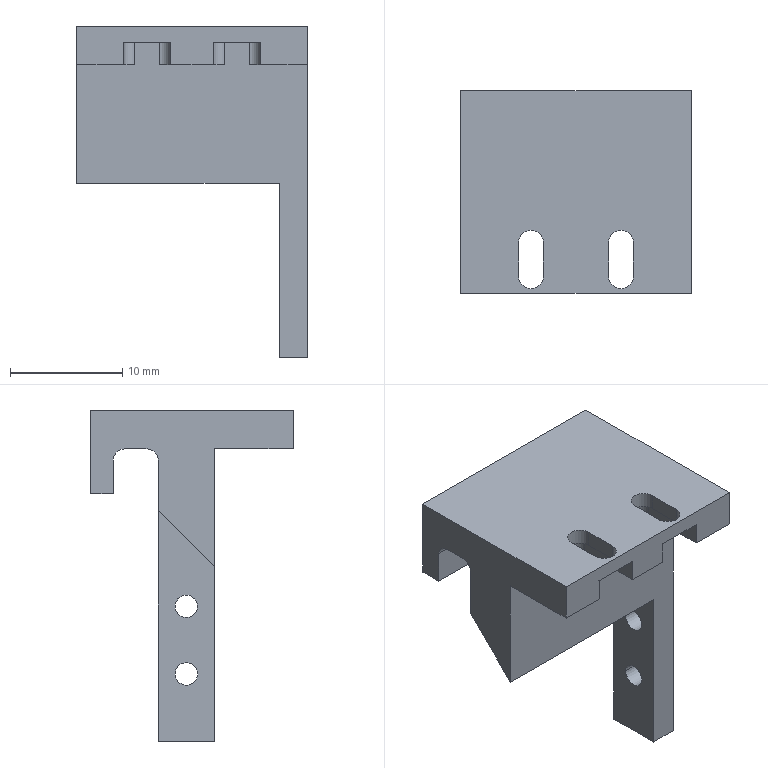NC program | NX | posted with a generic post | part box 20.5 x 18 x 29.4 mm
Lines 1922 to 2950 of 6588:
(CAVITY_MILL_COPY_COPY , TOOL : D2)
N3830 T02 M6
N3832 G54
N3834 G17 G0 G90 X-3.982 Y0.408 S7500 M3
N3836 G43 Z30. H2
N3838 Z-14.1
N3840 G94 G1 Z-15.6 F1000.
N3842 X-4.3 Y0.323
N3844 G2 X-5.266 Y0.581 R1.
N3846 X-6.258 Y2.485 R3.56 F850.
N3848 G3 X-6.75 Y2.899 R0.5
N3850 G1 Y-0.9
N3852 X-2.946
N3854 G3 X-3.361 Y-0.407 R0.5
N3856 G2 X-5.266 Y0.581 R3.56
N3858 X-5.526 Y1.547 R1.
N3860 G1 X-5.441 Y1.865
N3862 Z-14.1
N3864 G0 X-3.931 Y0.484 Z-14.2
N3866 G1 Z-15.7 F1000.
N3868 X-4.247 Y0.392
N3870 G2 X-5.218 Y0.631 R1.
N3872 X-6.258 Y2.57 R3.56 F850.
N3874 G3 X-6.75 Y2.982 R0.5
N3876 G1 Y-0.8
N3878 X-2.949
N3880 G3 X-3.364 Y-0.307 R0.5
N3882 G2 X-5.218 Y0.631 R3.56
N3884 X-5.497 Y1.591 R1.
N3886 G1 X-5.419 Y1.911
N3888 Z-14.2
N3890 G0 X-3.881 Y0.561 Z-14.3
N3892 G1 Z-15.8 F1000.
N3894 X-4.196 Y0.463
N3896 G2 X-5.171 Y0.682 R1.
N3898 X-6.258 Y2.646 R3.56 F850.
N3900 G3 X-6.751 Y3.055 R0.5
N3902 G1 X-6.75 Y3.
N3904 Y-0.7
N3906 X-2.954
N3908 G3 X-3.369 Y-0.207 R0.5
N3910 G2 X-5.171 Y0.682 R3.56
N3912 X-5.469 Y1.637 R1.
N3914 G1 X-5.397 Y1.958
N3916 Z-14.3
N3918 G0 X-3.833 Y0.639 Z-14.4
N3920 G1 Z-15.9 F1000.
N3922 X-4.145 Y0.535
N3924 G2 X-5.125 Y0.734 R1.
N3926 X-6.259 Y2.714 R3.56 F850.
N3928 G3 X-6.757 Y3.118 R0.5
N3930 G1 X-6.75 Y3.
N3932 Y-0.6
N3934 X-2.961
N3936 G3 X-3.376 Y-0.107 R0.5
N3938 G2 X-5.125 Y0.734 R3.56
N3940 X-5.443 Y1.682 R1.
N3942 G1 X-5.377 Y2.005
N3944 Z-14.4
N3946 G0 X-3.786 Y0.718 Z-14.5
N3948 G1 Z-16. F1000.
N3950 X-4.097 Y0.607
N3952 G2 X-5.08 Y0.787 R1.
N3954 X-6.26 Y2.775 R3.56 F850.
N3956 G3 X-6.765 Y3.173 R0.5
N3958 G1 X-6.75 Y3.
N3960 Y-0.5
N3962 X-2.97
N3964 G3 X-3.385 Y-0.007 R0.5
N3966 G2 X-5.08 Y0.787 R3.56
N3968 X-5.416 Y1.729 R1.
N3970 G1 X-5.357 Y2.053
N3972 Z-14.5
N3974 G0 X-3.741 Y0.798 Z-14.6
N3976 G1 Z-16.1 F1000.
N3978 X-4.049 Y0.681
N3980 G2 X-5.036 Y0.841 R1.
N3982 X-6.262 Y2.83 R3.56 F850.
N3984 G3 X-6.775 Y3.221 R0.5
N3986 G2 X-6.75 Y3. R1.
N3988 G1 Y-0.4
N3990 X-2.982
N3992 G3 X-3.396 Y0.093 R0.5
N3994 G2 X-5.036 Y0.841 R3.56
N3996 X-5.391 Y1.776 R1.
N3998 G1 X-5.339 Y2.101
N4000 Z-14.6
N4002 G0 X-3.697 Y0.88 Z-14.7
N4004 G1 Z-16.2 F1000.
N4006 X-4.003 Y0.756
N4008 G2 X-4.993 Y0.896 R1.
N4010 X-6.263 Y2.88 R3.56 F850.
N4012 G3 X-6.785 Y3.263 R0.5
N4014 G2 X-6.75 Y3. R1.
N4016 G1 Y-0.3
N4018 X-2.995
N4020 G3 X-3.409 Y0.193 R0.5
N4022 G2 X-4.993 Y0.896 R3.56
N4024 X-5.367 Y1.824 R1.
N4026 G1 X-5.321 Y2.15
N4028 Z-14.7
N4030 G0 X-3.655 Y0.962 Z-14.8
N4032 G1 Z-16.3 F1000.
N4034 X-3.958 Y0.833
N4036 G2 X-4.951 Y0.952 R1.
N4038 X-6.265 Y2.925 R3.56 F850.
N4040 G3 X-6.796 Y3.3 R0.5
N4042 G2 X-6.75 Y3. R1.
N4044 G1 Y-0.2
N4046 X-3.01
N4048 G3 X-3.424 Y0.293 R0.5
N4050 G2 X-4.951 Y0.952 R3.56
N4052 X-5.344 Y1.872 R1.
N4054 G1 X-5.304 Y2.199
N4056 Z-14.8
N4058 G0 X-3.615 Y1.045 Z-14.9
N4060 G1 Z-16.4 F1000.
N4062 X-3.915 Y0.91
N4064 G2 X-4.91 Y1.01 R1.
N4066 X-6.267 Y2.968 R3.56 F850.
N4068 G3 X-6.807 Y3.334 R0.5
N4070 G2 X-6.75 Y3. R1.
N4072 G1 Y-0.1
N4074 X-3.027
N4076 G3 X-3.441 Y0.393 R0.5
N4078 G2 X-4.91 Y1.01 R3.56
N4080 X-5.321 Y1.921 R1.
N4082 G1 X-5.288 Y2.249
N4084 Z-14.9
N4086 G0 X-3.576 Y1.13 Z-15.
N4088 G1 Z-16.5 F1000.
N4090 X-3.873 Y0.988
N4092 G2 X-4.87 Y1.068 R1.
N4094 X-6.27 Y3.007 R3.56 F850.
N4096 G3 X-6.818 Y3.363 R0.5
N4098 G2 X-6.75 Y3. R1.
N4100 G1 Y0.
N4102 X-3.046
N4104 G3 X-3.461 Y0.493 R0.5
N4106 G2 X-4.87 Y1.068 R3.56
N4108 X-5.3 Y1.971 R1.
N4110 G1 X-5.273 Y2.299
N4112 Z-15.
N4114 G0 X-3.538 Y1.216 Z-15.1
N4116 G1 Z-16.6 F1000.
N4118 X-3.833 Y1.068
N4120 G2 X-4.831 Y1.127 R1.
N4122 X-6.272 Y3.045 R3.56 F850.
N4124 G3 X-6.829 Y3.39 R0.5
N4126 G2 X-6.75 Y3. R1.
N4128 G1 Y0.1
N4130 X-3.068
N4132 G3 X-3.482 Y0.593 R0.5
N4134 G2 X-4.831 Y1.127 R3.56
N4136 X-5.279 Y2.021 R1.
N4138 G1 X-5.26 Y2.35
N4140 Z-15.1
N4142 G0 X-3.502 Y1.303 Z-15.2
N4144 G1 Z-16.7 F1000.
N4146 X-3.794 Y1.149
N4148 G2 X-4.793 Y1.187 R1.
N4150 X-6.275 Y3.08 R3.56 F850.
N4152 G3 X-6.84 Y3.415 R0.5
N4154 G2 X-6.75 Y3. R1.
N4156 G1 Y0.2
N4158 X-3.092
N4160 G3 X-3.506 Y0.693 R0.5
N4162 G2 X-4.793 Y1.187 R3.56
N4164 X-5.259 Y2.072 R1.
N4166 G1 X-5.247 Y2.401
N4168 Z-15.2
N4170 G0 X-3.468 Y1.391 Z-15.3
N4172 G1 Z-16.8 F1000.
N4174 X-3.756 Y1.231
N4176 G2 X-4.756 Y1.249 R1.
N4178 X-6.279 Y3.114 R3.56 F850.
N4180 G3 X-6.851 Y3.437 R0.5
N4182 G2 X-6.75 Y3. R1.
N4184 G1 Y0.3
N4186 X-3.117
N4188 G3 X-3.532 Y0.793 R0.5
N4190 G2 X-4.756 Y1.249 R3.56
N4192 X-5.241 Y2.123 R1.
N4194 G1 X-5.235 Y2.453
N4196 Z-15.3
N4198 G0 X-3.436 Y1.48 Z-15.4
N4200 G1 Z-16.9 F1000.
N4202 X-3.72 Y1.314
N4204 G2 X-4.72 Y1.311 R1.
N4206 X-6.282 Y3.147 R3.56 F850.
N4208 G3 X-6.861 Y3.458 R0.5
N4210 G2 X-6.75 Y3. R1.
N4212 G1 Y0.4
N4214 X-3.145
N4216 G3 X-3.56 Y0.893 R0.5
N4218 G2 X-4.72 Y1.311 R3.56
N4220 X-5.223 Y2.176 R1.
N4222 G1 X-5.224 Y2.505
N4224 Z-15.4
N4226 G0 X-3.41 Y1.567 Z-15.5
N4228 G1 Z-17. F1000.
N4230 X-3.686 Y1.399
N4232 G2 X-4.685 Y1.375 R1.
N4234 X-6.286 Y3.178 R3.56 F850.
N4236 G3 X-6.871 Y3.477 R0.5
N4238 G2 X-6.75 Y3. R1.
N4240 G1 Y0.5
N4242 X-3.176
N4244 G3 X-3.59 Y0.993 R0.5
N4246 G2 X-4.685 Y1.375 R3.56
N4248 X-5.206 Y2.229 R1.
N4250 G1 X-5.214 Y2.558
N4252 Z-15.5
N4254 G0 X-3.39 Y1.653 Z-15.6
N4256 G1 Z-17.1 F1000.
N4258 X-3.653 Y1.485
N4260 G2 X-4.652 Y1.44 R1.
N4262 X-6.29 Y3.209 R3.56 F850.
N4264 G3 X-6.882 Y3.496 R0.5
N4266 G2 X-6.75 Y3. R1.
N4268 G1 Y0.6
N4270 X-3.208
N4272 G3 X-3.623 Y1.093 R0.5
N4274 G2 X-4.652 Y1.44 R3.56
N4276 X-5.19 Y2.282 R1.
N4278 G1 X-5.205 Y2.611
N4280 Z-15.6
N4282 G0 X-3.376 Y1.737 Z-15.7
N4284 G1 Z-17.2 F1000.
N4286 X-3.622 Y1.572
N4288 G2 X-4.619 Y1.506 R1.
N4290 X-6.295 Y3.24 R3.56 F850.
N4292 G3 X-6.892 Y3.514 R0.5
N4294 G2 X-6.75 Y3. R1.
N4296 G1 Y0.7
N4298 X-3.243
N4300 G3 X-3.658 Y1.193 R0.5
N4302 G2 X-4.619 Y1.506 R3.56
N4304 X-5.176 Y2.337 R1.
N4306 G1 X-5.198 Y2.665
N4308 Z-15.7
N4310 G0 X-3.366 Y1.819 Z-15.8
N4312 G1 Z-17.3 F1000.
N4314 X-3.592 Y1.66
N4316 G2 X-4.588 Y1.573 R1.
N4318 X-6.3 Y3.271 R3.56 F850.
N4320 G3 X-6.903 Y3.532 R0.5
N4322 G2 X-6.75 Y3. R1.
N4324 G1 Y0.8
N4326 X-3.281
N4328 G3 X-3.695 Y1.293 R0.5
N4330 G2 X-4.588 Y1.573 R3.56
N4332 X-5.162 Y2.392 R1.
N4334 G1 X-5.191 Y2.72
N4336 Z-15.8
N4338 G0 X-3.361 Y1.899 Z-15.9
N4340 G1 Z-17.4 F1000.
N4342 X-3.564 Y1.75
N4344 G2 X-4.558 Y1.641 R1.
N4346 X-6.306 Y3.302 R3.56 F850.
N4348 G3 X-6.915 Y3.55 R0.5
N4350 G2 X-6.75 Y3. R1.
N4352 G1 Y0.9
N4354 X-3.32
N4356 G3 X-3.735 Y1.393 R0.5
N4358 G2 X-4.558 Y1.641 R3.56
N4360 X-5.15 Y2.447 R1.
N4362 G1 X-5.185 Y2.775
N4364 Z-15.9
N4366 G0 X-3.36 Y1.978 Z-16.
N4368 G1 Z-17.5 F1000.
N4370 X-3.538 Y1.841
N4372 G2 X-4.529 Y1.711 R1.
N4374 X-6.313 Y3.333 R3.56 F850.
N4376 G3 X-6.927 Y3.568 R0.5
N4378 G2 X-6.75 Y3. R1.
N4380 G1 Y1.
N4382 X-3.363
N4384 G3 X-3.777 Y1.493 R0.5
N4386 G2 X-4.529 Y1.711 R3.56
N4388 X-5.138 Y2.504 R1.
N4390 G1 X-5.181 Y2.831
N4392 Z-16.
N4394 G0 X-3.362 Y2.055 Z-16.1
N4396 G1 Z-17.6 F1000.
N4398 X-3.513 Y1.934
N4400 G2 X-4.502 Y1.782 R1.
N4402 X-6.321 Y3.365 R3.56 F850.
N4404 G3 X-6.94 Y3.586 R0.5
N4406 G2 X-6.75 Y3. R1.
N4408 G1 Y1.1
N4410 X-3.408
N4412 G3 X-3.822 Y1.593 R0.5
N4414 G2 X-4.502 Y1.782 R3.56
N4416 X-5.128 Y2.561 R1.
N4418 G1 X-5.178 Y2.887
N4420 Z-16.1
N4422 G0 X-3.369 Y2.131 Z-16.2
N4424 G1 Z-17.7 F1000.
N4426 X-3.491 Y2.028
N4428 G2 X-4.475 Y1.854 R1.
N4430 X-6.329 Y3.396 R3.56 F850.
N4432 G3 X-6.953 Y3.604 R0.5
N4434 G2 X-6.75 Y3. R1.
N4436 G1 Y1.2
N4438 X-3.455
N4440 G3 X-3.87 Y1.693 R0.5
N4442 G2 X-4.475 Y1.854 R3.56
N4444 X-5.119 Y2.62 R1.
N4446 G1 X-5.176 Y2.944
N4448 Z-16.2
N4450 G0 X-3.379 Y2.204 Z-16.3
N4452 G1 Z-17.8 F1000.
N4454 X-3.47 Y2.124
N4456 G2 X-4.45 Y1.927 R1.
N4458 X-6.338 Y3.428 R3.56 F850.
N4460 G3 X-6.967 Y3.622 R0.5
N4462 G2 X-6.75 Y3. R1.
N4464 G1 Y1.3
N4466 X-3.506
N4468 G3 X-3.92 Y1.793 R0.5
N4470 G2 X-4.45 Y1.927 R3.56
N4472 X-5.111 Y2.679 R1.
N4474 G1 X-5.175 Y3.001
N4476 Z-16.3
N4478 G0 X-3.392 Y2.275 Z-16.4
N4480 G1 Z-17.9 F1000.
N4482 X-3.451 Y2.221
N4484 G2 X-4.427 Y2.003 R1.
N4486 X-6.348 Y3.46 R3.56 F850.
N4488 G3 X-6.981 Y3.639 R0.5
N4490 G2 X-6.75 Y3. R1.
N4492 G1 Y1.4
N4494 X-3.559
N4496 G3 X-3.973 Y1.893 R0.5
N4498 G2 X-4.427 Y2.003 R3.56
N4500 X-5.104 Y2.738 R1.
N4502 G1 X-5.176 Y3.06
N4504 Z-16.4
N4506 G0 X-3.41 Y2.344 Z-16.5
N4508 G1 Z-18. F1000.
N4510 X-3.434 Y2.32
N4512 G2 X-4.405 Y2.079 R1.
N4514 X-6.359 Y3.492 R3.56 F850.
N4516 G3 X-6.996 Y3.657 R0.5
N4518 G2 X-6.75 Y3. R1.
N4520 G1 Y1.5
N4522 X-3.615
N4524 G3 X-4.03 Y1.993 R0.5
N4526 G2 X-4.405 Y2.079 R3.56
N4528 X-5.099 Y2.799 R1.
N4530 G1 X-5.178 Y3.119
N4532 Z-16.5
N4534 G0 X-3.43 Y2.41 Z-16.6
N4536 G1 Z-18.1 F1000.
N4538 G2 X-4.384 Y2.157 R1.
N4540 X-6.371 Y3.524 R3.56 F850.
N4542 G3 X-7.011 Y3.674 R0.5
N4544 G2 X-6.75 Y3. R1.
N4546 G1 Y1.6
N4548 X-3.675
N4550 G3 X-4.089 Y2.093 R0.5
N4552 G2 X-4.384 Y2.157 R3.56
N4554 X-5.095 Y2.861 R1.
N4556 G1 X-5.182 Y3.179
N4558 Z-16.6
N4560 G0 X-3.456 Y2.475 Z-16.7
N4562 G1 Z-18.2 F1000.
N4564 G2 X-4.366 Y2.237 R1.
N4566 X-6.384 Y3.556 R3.56 F850.
N4568 G3 X-7.028 Y3.691 R0.5
N4570 G2 X-6.75 Y3. R1.
N4572 G1 Y1.7
N4574 X-3.737
N4576 G3 X-4.151 Y2.193 R0.5
N4578 G2 X-4.366 Y2.237 R3.56
N4580 X-5.092 Y2.923 R1.
N4582 G1 X-5.187 Y3.239
N4584 Z-16.7
N4586 G0 X-3.488 Y2.538 Z-16.8
N4588 G1 Z-18.3 F1000.
N4590 G2 X-4.348 Y2.318 R1.
N4592 X-6.398 Y3.589 R3.56 F850.
N4594 G3 X-7.044 Y3.709 R0.5
N4596 G2 X-6.75 Y3. R1.
N4598 G1 Y1.8
N4600 X-3.803
N4602 G3 X-4.217 Y2.293 R0.5
N4604 G1 X-4.348 Y2.318
N4606 G2 X-5.091 Y2.987 R1.
N4608 G1 X-5.193 Y3.3
N4610 Z-16.8
N4612 G0 X-3.525 Y2.602 Z-16.9
N4614 G1 Z-18.4 F1000.
N4616 G2 X-4.333 Y2.401 R1.
N4618 X-6.412 Y3.622 R3.56 F850.
N4620 G3 X-7.062 Y3.726 R0.5
N4622 G2 X-6.75 Y3. R1.
N4624 G1 Y1.9
N4626 X-3.872
N4628 G3 X-4.333 Y2.401 R0.502
N4630 G2 X-5.092 Y3.052 R1.
N4632 G1 X-5.201 Y3.363
N4634 Z-16.9
N4636 G0 X-3.503 Y2.6 Z-17.
N4638 G1 Z-18.5 F1000.
N4640 G2 X-4.31 Y2.481 R1.
N4642 G1 X-4.36 Y2.493 F850.
N4644 G2 X-6.428 Y3.655 R3.56
N4646 G3 X-7.08 Y3.742 R0.5
N4648 G2 X-6.75 Y3. R1.
N4650 G1 Y2.
N4652 X-3.945
N4654 G3 X-4.31 Y2.481 R0.5
N4656 G2 X-5.008 Y3.197 R1.
N4658 G1 X-5.044 Y3.338
N4660 Z-17.
N4662 G0 X-3.033 Y2.7 Z-17.1
N4664 G1 Z-18.6 F1000.
N4666 X-3.279 Y2.552
N4668 G2 X-4.279 Y2.537 R1.
N4670 G1 X-4.437 Y2.593 F850.
N4672 G2 X-6.445 Y3.688 R3.56
N4674 G3 X-7.099 Y3.759 R0.5
N4676 G2 X-6.75 Y3. R1.
N4678 G1 Y2.1
N4680 X-4.022
N4682 G3 X-4.279 Y2.537 R0.5
N4684 G2 X-4.787 Y3.3 R1.
N4686 G1 Z-17.1
N4688 G0 X-7.487 Y4.578 Z-17.2
N4690 G1 Z-18.7 F1000.
N4692 G3 X-7.119 Y3.776 R1.
N4694 G2 X-6.75 Y3. R1. F850.
N4696 G1 Y2.2
N4698 X-4.104
N4700 G3 X-3.238 Y2.7 R1.
N4702 G1 X-3.18 Y2.8
N4704 Z-17.2
N4706 G0 X-7.529 Y4.585 Z-17.3
N4708 G1 Z-18.8 F1000.
N4710 G3 X-7.139 Y3.792 R1.
N4712 G2 X-6.75 Y3. R1. F850.
N4714 G1 Y2.3
N4716 X-4.189
N4718 G3 X-3.323 Y2.8 R1.
N4720 G1 X-3.265 Y2.9
N4722 Z-17.3
N4724 G0 X-7.571 Y4.59 Z-17.4
N4726 G1 Z-18.9 F1000.
N4728 G3 X-7.161 Y3.808 R1.
N4730 G2 X-6.75 Y3. R1. F850.
N4732 G1 Y2.4
N4734 X-4.279
N4736 G3 X-3.413 Y2.9 R1.
N4738 G1 X-3.356 Y3.
N4740 Z-17.4
N4742 G0 X-7.615 Y4.594 Z-17.5
N4744 G1 Z-19. F1000.
N4746 G3 X-7.183 Y3.824 R1.
N4748 G2 X-6.75 Y3. R1. F850.
N4750 G1 Y2.5
N4752 X-4.375
N4754 G3 X-3.509 Y3. R1.
N4756 G1 X-3.451 Y3.1
N4758 Z-17.5
N4760 G0 X-7.661 Y4.598 Z-17.6
N4762 G1 Z-19.1 F1000.
N4764 G3 X-7.207 Y3.84 R1.
N4766 G2 X-6.75 Y3. R1. F850.
N4768 G1 Y2.6
N4770 X-4.476
N4772 G3 X-3.61 Y3.1 R1.
N4774 G1 X-3.552 Y3.2
N4776 Z-17.6
N4778 G0 X-7.708 Y4.599 Z-17.7
N4780 G1 Z-19.2 F1000.
N4782 G3 X-7.232 Y3.855 R1.
N4784 G2 X-6.75 Y3. R1. F850.
N4786 G1 Y2.7
N4788 X-4.582
N4790 G3 X-3.716 Y3.2 R1.
N4792 G1 X-3.659 Y3.3
N4794 Z-17.7
N4796 G0 X-7.756 Y4.6 Z-17.8
N4798 G1 Z-19.3 F1000.
N4800 G3 X-7.258 Y3.871 R1.
N4802 G2 X-6.75 Y3. R1. F850.
N4804 G1 Y2.8
N4806 X-4.696
N4808 G3 X-3.83 Y3.3 R1.
N4810 G1 X-3.772 Y3.4
N4812 Z-17.8
N4814 G0 X-7.806 Y4.6 Z-17.9
N4816 G1 Z-19.4 F1000.
N4818 G3 X-7.286 Y3.886 R1.
N4820 G2 X-6.75 Y3. R1. F850.
N4822 G1 Y2.9
N4824 X-4.817
N4826 G3 X-3.95 Y3.4 R1.
N4828 G1 X-3.893 Y3.5
N4830 Z-17.9
N4832 G0 X-7.859 Y4.6 Z-18.
N4834 G1 Z-19.5 F1000.
N4836 G3 X-7.315 Y3.9 R1.
N4838 G2 X-6.75 Y3. R1. F850.
N4840 G1 X-4.945
N4842 G3 X-4.079 Y3.5 R1.
N4844 G1 X-4.022 Y3.6
N4846 Z-18.
N4848 G0 X-7.915 Y4.6 Z-18.1
N4850 G1 Z-19.6 F1000.
N4852 G3 X-7.346 Y3.915 R1.
N4854 G2 X-6.755 Y3.1 R1. F850.
N4856 G1 X-5.084
N4858 G3 X-4.218 Y3.6 R1.
N4860 G1 X-4.16 Y3.7
N4862 Z-18.1
N4864 G0 X-7.974 Y4.6 Z-18.2
N4866 G1 Z-19.7 F1000.
N4868 G3 X-7.379 Y3.929 R1.
N4870 G2 X-6.77 Y3.2 R1. F850.
N4872 G1 X-5.232
N4874 G3 X-4.366 Y3.7 R1.
N4876 G1 X-4.309 Y3.8
N4878 Z-18.2
N4880 G0 X-8.037 Y4.6 Z-18.3
N4882 G1 Z-19.8 F1000.
N4884 G3 X-7.414 Y3.942 R1.
N4886 G2 X-6.796 Y3.3 R1. F850.
N4888 G1 X-5.394
N4890 G3 X-4.528 Y3.8 R1.
N4892 G1 X-4.47 Y3.9
N4894 Z-18.3
N4896 G0 X-8.106 Y4.6 Z-18.4
N4898 G1 Z-19.9 F1000.
N4900 G3 X-7.453 Y3.955 R1.
N4902 G2 X-6.833 Y3.4 R1. F850.
N4904 G1 X-5.571
N4906 G3 X-4.705 Y3.9 R1.
N4908 G1 X-4.647 Y4.
N4910 Z-18.4
N4912 G0 X-8.182 Y4.6 Z-18.5
N4914 G1 Z-20. F1000.
N4916 G3 X-7.495 Y3.967 R1.
N4918 G2 X-6.884 Y3.5 R1. F850.
N4920 G1 X-5.766
N4922 G3 X-4.9 Y4. R1.
N4924 G1 X-4.842 Y4.1
N4926 Z-18.5
N4928 G0 X-8.268 Y4.6 Z-18.6
N4930 G1 Z-20.1 F1000.
N4932 G3 X-7.542 Y3.978 R1.
N4934 G2 X-6.95 Y3.6 R1. F850.
N4936 G1 X-5.986
N4938 G3 X-5.12 Y4.1 R1.
N4940 G1 X-5.062 Y4.2
N4942 Z-18.6
N4944 G0 X-8.368 Y4.6 Z-18.7
N4946 G1 Z-20.2 F1000.
N4948 G3 X-7.596 Y3.988 R1.
N4950 G2 X-7.036 Y3.7 R1. F850.
N4952 G1 X-6.24
N4954 G3 X-5.374 Y4.2 R1.
N4956 G1 X-5.316 Y4.3
N4958 Z-18.7
N4960 G0 X-8.489 Y4.6 Z-18.8
N4962 G1 Z-20.3 F1000.
N4964 X-8.477 Y4.572
N4966 G3 X-7.659 Y3.996 R1.
N4968 G2 X-7.15 Y3.8 R1. F850.
N4970 G1 X-6.545
N4972 G3 X-5.679 Y4.3 R1.
N4974 G1 X-5.622 Y4.4
N4976 Z-18.8
N4978 G0 Z30.
N4980 X-12.055 Y3.971
N4982 Z-20.6
N4984 G1 Z-22.1 F1000.
N4986 X-11.773 Y4.134
N4988 G3 X-11.273 Y5. R1.
N4990 G1 X-10.373
N4992 X-10.374 Y4.896 F850.
N4994 X-10.25 Y4.9
N4996 X10.25
N4998 X10.374 Y4.896
N5000 G2 X10.374 Y5.104 R4.46
N5002 G1 X10.25 Y5.1
N5004 X-10.25
N5006 X-10.374 Y5.104
N5008 X-10.373 Y5.
N5010 X-11.273
N5012 G2 X-11.471 Y3.827 R3.56
N5014 G3 X-11.226 Y3.217 R0.5
N5016 G2 X-10.25 Y4. R1.
N5018 G1 X10.25
N5020 G2 X11.226 Y3.217 R1.
N5022 G3 X11.471 Y3.827 R0.5
N5024 G2 X11.471 Y6.173 R3.56
N5026 G3 X11.226 Y6.783 R0.5
N5028 G2 X10.25 Y6. R1.
N5030 G1 X-10.25
N5032 G2 X-11.226 Y6.783 R1.
N5034 G3 X-11.471 Y6.173 R0.5
N5036 G2 X-11.273 Y5. R3.56
N5038 X-11.773 Y4.134 R1.
N5040 G1 X-12.055 Y3.971
N5042 Z-20.6
N5044 G0 Z-20.7
N5046 G1 Z-22.2 F1000.
N5048 X-11.773 Y4.134
N5050 G3 X-11.273 Y5. R1.
N5052 G1 X-10.373
N5054 X-10.374 Y4.896 F850.
N5056 X-10.25 Y4.9
N5058 X10.25
N5060 X10.374 Y4.896
N5062 G2 X10.374 Y5.104 R4.46
N5064 G1 X10.25 Y5.1
N5066 X-10.25
N5068 X-10.374 Y5.104
N5070 X-10.373 Y5.
N5072 X-11.273
N5074 G2 X-11.471 Y3.827 R3.56
N5076 G3 X-11.226 Y3.217 R0.5
N5078 G2 X-10.25 Y4. R1.
N5080 G1 X10.25
N5082 G2 X11.226 Y3.217 R1.
N5084 G3 X11.471 Y3.827 R0.5
N5086 G2 X11.471 Y6.173 R3.56
N5088 G3 X11.226 Y6.783 R0.5
N5090 G2 X10.25 Y6. R1.
N5092 G1 X-10.25
N5094 G2 X-11.226 Y6.783 R1.
N5096 G3 X-11.471 Y6.173 R0.5
N5098 G2 X-11.273 Y5. R3.56
N5100 X-11.773 Y4.134 R1.
N5102 G1 X-12.055 Y3.971
N5104 Z-20.7
N5106 G0 Z-20.8
N5108 G1 Z-22.3 F1000.
N5110 X-11.773 Y4.134
N5112 G3 X-11.273 Y5. R1.
N5114 G1 X-10.373
N5116 X-10.374 Y4.896 F850.
N5118 X-10.25 Y4.9
N5120 X10.25
N5122 X10.374 Y4.896
N5124 G2 X10.374 Y5.104 R4.46
N5126 G1 X10.25 Y5.1
N5128 X-10.25
N5130 X-10.374 Y5.104
N5132 X-10.373 Y5.
N5134 X-11.273
N5136 G2 X-11.471 Y3.827 R3.56
N5138 G3 X-11.226 Y3.217 R0.5
N5140 G2 X-10.25 Y4. R1.
N5142 G1 X10.25
N5144 G2 X11.226 Y3.217 R1.
N5146 G3 X11.471 Y3.827 R0.5
N5148 G2 X11.471 Y6.173 R3.56
N5150 G3 X11.226 Y6.783 R0.5
N5152 G2 X10.25 Y6. R1.
N5154 G1 X-10.25
N5156 G2 X-11.226 Y6.783 R1.
N5158 G3 X-11.471 Y6.173 R0.5
N5160 G2 X-11.273 Y5. R3.56
N5162 X-11.773 Y4.134 R1.
N5164 G1 X-12.055 Y3.971
N5166 Z-20.8
N5168 G0 Z-20.9
N5170 G1 Z-22.4 F1000.
N5172 X-11.773 Y4.134
N5174 G3 X-11.273 Y5. R1.
N5176 G1 X-10.373
N5178 X-10.374 Y4.896 F850.
N5180 X-10.25 Y4.9
N5182 X10.25
N5184 X10.374 Y4.896
N5186 G2 X10.374 Y5.104 R4.46
N5188 G1 X10.25 Y5.1
N5190 X-10.25
N5192 X-10.374 Y5.104
N5194 X-10.373 Y5.
N5196 X-11.273
N5198 G2 X-11.471 Y3.827 R3.56
N5200 G3 X-11.226 Y3.217 R0.5
N5202 G2 X-10.25 Y4. R1.
N5204 G1 X10.25
N5206 G2 X11.226 Y3.217 R1.
N5208 G3 X11.471 Y3.827 R0.5
N5210 G2 X11.471 Y6.173 R3.56
N5212 G3 X11.226 Y6.783 R0.5
N5214 G2 X10.25 Y6. R1.
N5216 G1 X-10.25
N5218 G2 X-11.226 Y6.783 R1.
N5220 G3 X-11.471 Y6.173 R0.5
N5222 G2 X-11.273 Y5. R3.56
N5224 X-11.773 Y4.134 R1.
N5226 G1 X-12.055 Y3.971
N5228 Z-20.9
N5230 G0 Z-21.
N5232 G1 Z-22.5 F1000.
N5234 X-11.773 Y4.134
N5236 G3 X-11.273 Y5. R1.
N5238 G1 X-10.373
N5240 X-10.374 Y4.896 F850.
N5242 X-10.25 Y4.9
N5244 X10.25
N5246 X10.374 Y4.896
N5248 G2 X10.374 Y5.104 R4.46
N5250 G1 X10.25 Y5.1
N5252 X-10.25
N5254 X-10.374 Y5.104
N5256 X-10.373 Y5.
N5258 X-11.273
N5260 G2 X-11.471 Y3.827 R3.56
N5262 G3 X-11.226 Y3.217 R0.5
N5264 G2 X-10.25 Y4. R1.
N5266 G1 X10.25
N5268 G2 X11.226 Y3.217 R1.
N5270 G3 X11.471 Y3.827 R0.5
N5272 G2 X11.471 Y6.173 R3.56
N5274 G3 X11.226 Y6.783 R0.5
N5276 G2 X10.25 Y6. R1.
N5278 G1 X-10.25
N5280 G2 X-11.226 Y6.783 R1.
N5282 G3 X-11.471 Y6.173 R0.5
N5284 G2 X-11.273 Y5. R3.56
N5286 X-11.773 Y4.134 R1.
N5288 G1 X-12.055 Y3.971
N5290 Z-21.
N5292 G0 Z-21.1
N5294 G1 Z-22.6 F1000.
N5296 X-11.773 Y4.134
N5298 G3 X-11.273 Y5. R1.
N5300 G1 X-10.373
N5302 X-10.374 Y4.896 F850.
N5304 X-10.25 Y4.9
N5306 X10.25
N5308 X10.374 Y4.896
N5310 G2 X10.374 Y5.104 R4.46
N5312 G1 X10.25 Y5.1
N5314 X-10.25
N5316 X-10.374 Y5.104
N5318 X-10.373 Y5.
N5320 X-11.273
N5322 G2 X-11.471 Y3.827 R3.56
N5324 G3 X-11.226 Y3.217 R0.5
N5326 G2 X-10.25 Y4. R1.
N5328 G1 X10.25
N5330 G2 X11.226 Y3.217 R1.
N5332 G3 X11.471 Y3.827 R0.5
N5334 G2 X11.471 Y6.173 R3.56
N5336 G3 X11.226 Y6.783 R0.5
N5338 G2 X10.25 Y6. R1.
N5340 G1 X-10.25
N5342 G2 X-11.226 Y6.783 R1.
N5344 G3 X-11.471 Y6.173 R0.5
N5346 G2 X-11.273 Y5. R3.56
N5348 X-11.773 Y4.134 R1.
N5350 G1 X-12.055 Y3.971
N5352 Z-21.1
N5354 G0 Z-21.2
N5356 G1 Z-22.7 F1000.
N5358 X-11.773 Y4.134
N5360 G3 X-11.273 Y5. R1.
N5362 G1 X-10.373
N5364 X-10.374 Y4.896 F850.
N5366 X-10.25 Y4.9
N5368 X10.25
N5370 X10.374 Y4.896
N5372 G2 X10.374 Y5.104 R4.46
N5374 G1 X10.25 Y5.1
N5376 X-10.25
N5378 X-10.374 Y5.104
N5380 X-10.373 Y5.
N5382 X-11.273
N5384 G2 X-11.471 Y3.827 R3.56
N5386 G3 X-11.226 Y3.217 R0.5
N5388 G2 X-10.25 Y4. R1.
N5390 G1 X10.25
N5392 G2 X11.226 Y3.217 R1.
N5394 G3 X11.471 Y3.827 R0.5
N5396 G2 X11.471 Y6.173 R3.56
N5398 G3 X11.226 Y6.783 R0.5
N5400 G2 X10.25 Y6. R1.
N5402 G1 X-10.25
N5404 G2 X-11.226 Y6.783 R1.
N5406 G3 X-11.471 Y6.173 R0.5
N5408 G2 X-11.273 Y5. R3.56
N5410 X-11.773 Y4.134 R1.
N5412 G1 X-12.055 Y3.971
N5414 Z-21.2
N5416 G0 Z-21.3
N5418 G1 Z-22.8 F1000.
N5420 X-11.773 Y4.134
N5422 G3 X-11.273 Y5. R1.
N5424 G1 X-10.373
N5426 X-10.374 Y4.896 F850.
N5428 X-10.25 Y4.9
N5430 X10.25
N5432 X10.374 Y4.896
N5434 G2 X10.374 Y5.104 R4.46
N5436 G1 X10.25 Y5.1
N5438 X-10.25
N5440 X-10.374 Y5.104
N5442 X-10.373 Y5.
N5444 X-11.273
N5446 G2 X-11.471 Y3.827 R3.56
N5448 G3 X-11.226 Y3.217 R0.5
N5450 G2 X-10.25 Y4. R1.
N5452 G1 X10.25
N5454 G2 X11.226 Y3.217 R1.
N5456 G3 X11.471 Y3.827 R0.5
N5458 G2 X11.471 Y6.173 R3.56
N5460 G3 X11.226 Y6.783 R0.5
N5462 G2 X10.25 Y6. R1.
N5464 G1 X-10.25
N5466 G2 X-11.226 Y6.783 R1.
N5468 G3 X-11.471 Y6.173 R0.5
N5470 G2 X-11.273 Y5. R3.56
N5472 X-11.773 Y4.134 R1.
N5474 G1 X-12.055 Y3.971
N5476 Z-21.3
N5478 G0 Z-21.4
N5480 G1 Z-22.9 F1000.
N5482 X-11.773 Y4.134
N5484 G3 X-11.273 Y5. R1.
N5486 G1 X-10.373
N5488 X-10.374 Y4.896 F850.
N5490 X-10.25 Y4.9
N5492 X10.25
N5494 X10.374 Y4.896
N5496 G2 X10.374 Y5.104 R4.46
N5498 G1 X10.25 Y5.1
N5500 X-10.25
N5502 X-10.374 Y5.104
N5504 X-10.373 Y5.
N5506 X-11.273
N5508 G2 X-11.471 Y3.827 R3.56
N5510 G3 X-11.226 Y3.217 R0.5
N5512 G2 X-10.25 Y4. R1.
N5514 G1 X10.25
N5516 G2 X11.226 Y3.217 R1.
N5518 G3 X11.471 Y3.827 R0.5
N5520 G2 X11.471 Y6.173 R3.56
N5522 G3 X11.226 Y6.783 R0.5
N5524 G2 X10.25 Y6. R1.
N5526 G1 X-10.25
N5528 G2 X-11.226 Y6.783 R1.
N5530 G3 X-11.471 Y6.173 R0.5
N5532 G2 X-11.273 Y5. R3.56
N5534 X-11.773 Y4.134 R1.
N5536 G1 X-12.055 Y3.971
N5538 Z-21.4
N5540 G0 Z-21.5
N5542 G1 Z-23. F1000.
N5544 X-11.773 Y4.134
N5546 G3 X-11.273 Y5. R1.
N5548 G1 X-10.373
N5550 X-10.374 Y4.896 F850.
N5552 X-10.25 Y4.9
N5554 X10.25
N5556 X10.374 Y4.896
N5558 G2 X10.374 Y5.104 R4.46
N5560 G1 X10.25 Y5.1
N5562 X-10.25
N5564 X-10.374 Y5.104
N5566 X-10.373 Y5.
N5568 X-11.273
N5570 G2 X-11.471 Y3.827 R3.56
N5572 G3 X-11.226 Y3.217 R0.5
N5574 G2 X-10.25 Y4. R1.
N5576 G1 X10.25
N5578 G2 X11.226 Y3.217 R1.
N5580 G3 X11.471 Y3.827 R0.5
N5582 G2 X11.471 Y6.173 R3.56
N5584 G3 X11.226 Y6.783 R0.5
N5586 G2 X10.25 Y6. R1.
N5588 G1 X-10.25
N5590 G2 X-11.226 Y6.783 R1.
N5592 G3 X-11.471 Y6.173 R0.5
N5594 G2 X-11.273 Y5. R3.56
N5596 X-11.773 Y4.134 R1.
N5598 G1 X-12.055 Y3.971
N5600 Z-21.5
N5602 G0 Z-21.6
N5604 G1 Z-23.1 F1000.
N5606 X-11.773 Y4.134
N5608 G3 X-11.273 Y5. R1.
N5610 G1 X-10.373
N5612 X-10.374 Y4.896 F850.
N5614 X-10.25 Y4.9
N5616 X10.25
N5618 X10.374 Y4.896
N5620 G2 X10.374 Y5.104 R4.46
N5622 G1 X10.25 Y5.1
N5624 X-10.25
N5626 X-10.374 Y5.104
N5628 X-10.373 Y5.
N5630 X-11.273
N5632 G2 X-11.471 Y3.827 R3.56
N5634 G3 X-11.226 Y3.217 R0.5
N5636 G2 X-10.25 Y4. R1.
N5638 G1 X10.25
N5640 G2 X11.226 Y3.217 R1.
N5642 G3 X11.471 Y3.827 R0.5
N5644 G2 X11.471 Y6.173 R3.56
N5646 G3 X11.226 Y6.783 R0.5
N5648 G2 X10.25 Y6. R1.
N5650 G1 X-10.25
N5652 G2 X-11.226 Y6.783 R1.
N5654 G3 X-11.471 Y6.173 R0.5
N5656 G2 X-11.273 Y5. R3.56
N5658 X-11.773 Y4.134 R1.
N5660 G1 X-12.055 Y3.971
N5662 Z-21.6
N5664 G0 Z-21.7
N5666 G1 Z-23.2 F1000.
N5668 X-11.773 Y4.134
N5670 G3 X-11.273 Y5. R1.
N5672 G1 X-10.373
N5674 X-10.374 Y4.896 F850.
N5676 X-10.25 Y4.9
N5678 X10.25
N5680 X10.374 Y4.896
N5682 G2 X10.374 Y5.104 R4.46
N5684 G1 X10.25 Y5.1
N5686 X-10.25
N5688 X-10.374 Y5.104
N5690 X-10.373 Y5.
N5692 X-11.273
N5694 G2 X-11.471 Y3.827 R3.56
N5696 G3 X-11.226 Y3.217 R0.5
N5698 G2 X-10.25 Y4. R1.
N5700 G1 X10.25
N5702 G2 X11.226 Y3.217 R1.
N5704 G3 X11.471 Y3.827 R0.5
N5706 G2 X11.471 Y6.173 R3.56
N5708 G3 X11.226 Y6.783 R0.5
N5710 G2 X10.25 Y6. R1.
N5712 G1 X-10.25
N5714 G2 X-11.226 Y6.783 R1.
N5716 G3 X-11.471 Y6.173 R0.5
N5718 G2 X-11.273 Y5. R3.56
N5720 X-11.773 Y4.134 R1.
N5722 G1 X-12.055 Y3.971
N5724 Z-21.7
N5726 G0 Z-21.8
N5728 G1 Z-23.3 F1000.
N5730 X-11.773 Y4.134
N5732 G3 X-11.273 Y5. R1.
N5734 G1 X-10.373
N5736 X-10.374 Y4.896 F850.
N5738 X-10.25 Y4.9
N5740 X10.25
N5742 X10.374 Y4.896
N5744 G2 X10.374 Y5.104 R4.46
N5746 G1 X10.25 Y5.1
N5748 X-10.25
N5750 X-10.374 Y5.104
N5752 X-10.373 Y5.
N5754 X-11.273
N5756 G2 X-11.471 Y3.827 R3.56
N5758 G3 X-11.226 Y3.217 R0.5
N5760 G2 X-10.25 Y4. R1.
N5762 G1 X10.25
N5764 G2 X11.226 Y3.217 R1.
N5766 G3 X11.471 Y3.827 R0.5
N5768 G2 X11.471 Y6.173 R3.56
N5770 G3 X11.226 Y6.783 R0.5
N5772 G2 X10.25 Y6. R1.
N5774 G1 X-10.25
N5776 G2 X-11.226 Y6.783 R1.
N5778 G3 X-11.471 Y6.173 R0.5
N5780 G2 X-11.273 Y5. R3.56
N5782 X-11.773 Y4.134 R1.
N5784 G1 X-12.055 Y3.971
N5786 Z-21.8
N5788 G0 Z-21.9
N5790 G1 Z-23.4 F1000.
N5792 X-11.773 Y4.134
N5794 G3 X-11.273 Y5. R1.
N5796 G1 X-10.373
N5798 X-10.374 Y4.896 F850.
N5800 X-10.25 Y4.9
N5802 X10.25
N5804 X10.374 Y4.896
N5806 G2 X10.374 Y5.104 R4.46
N5808 G1 X10.25 Y5.1
N5810 X-10.25
N5812 X-10.374 Y5.104
N5814 X-10.373 Y5.
N5816 X-11.273
N5818 G2 X-11.471 Y3.827 R3.56
N5820 G3 X-11.226 Y3.217 R0.5
N5822 G2 X-10.25 Y4. R1.
N5824 G1 X10.25
N5826 G2 X11.226 Y3.217 R1.
N5828 G3 X11.471 Y3.827 R0.5
N5830 G2 X11.471 Y6.173 R3.56
N5832 G3 X11.226 Y6.783 R0.5
N5834 G2 X10.25 Y6. R1.
N5836 G1 X-10.25
N5838 G2 X-11.226 Y6.783 R1.
N5840 G3 X-11.471 Y6.173 R0.5
N5842 G2 X-11.273 Y5. R3.56
N5844 X-11.773 Y4.134 R1.
N5846 G1 X-12.055 Y3.971
N5848 Z-21.9
N5850 G0 Z-22.
N5852 G1 Z-23.5 F1000.
N5854 X-11.773 Y4.134
N5856 G3 X-11.273 Y5. R1.
N5858 G1 X-10.373
N5860 X-10.374 Y4.896 F850.
N5862 X-10.25 Y4.9
N5864 X10.25
N5866 X10.374 Y4.896
N5868 G2 X10.374 Y5.104 R4.46
N5870 G1 X10.25 Y5.1
N5872 X-10.25
N5874 X-10.374 Y5.104
N5876 X-10.373 Y5.
N5878 X-11.273
N5880 G2 X-11.471 Y3.827 R3.56